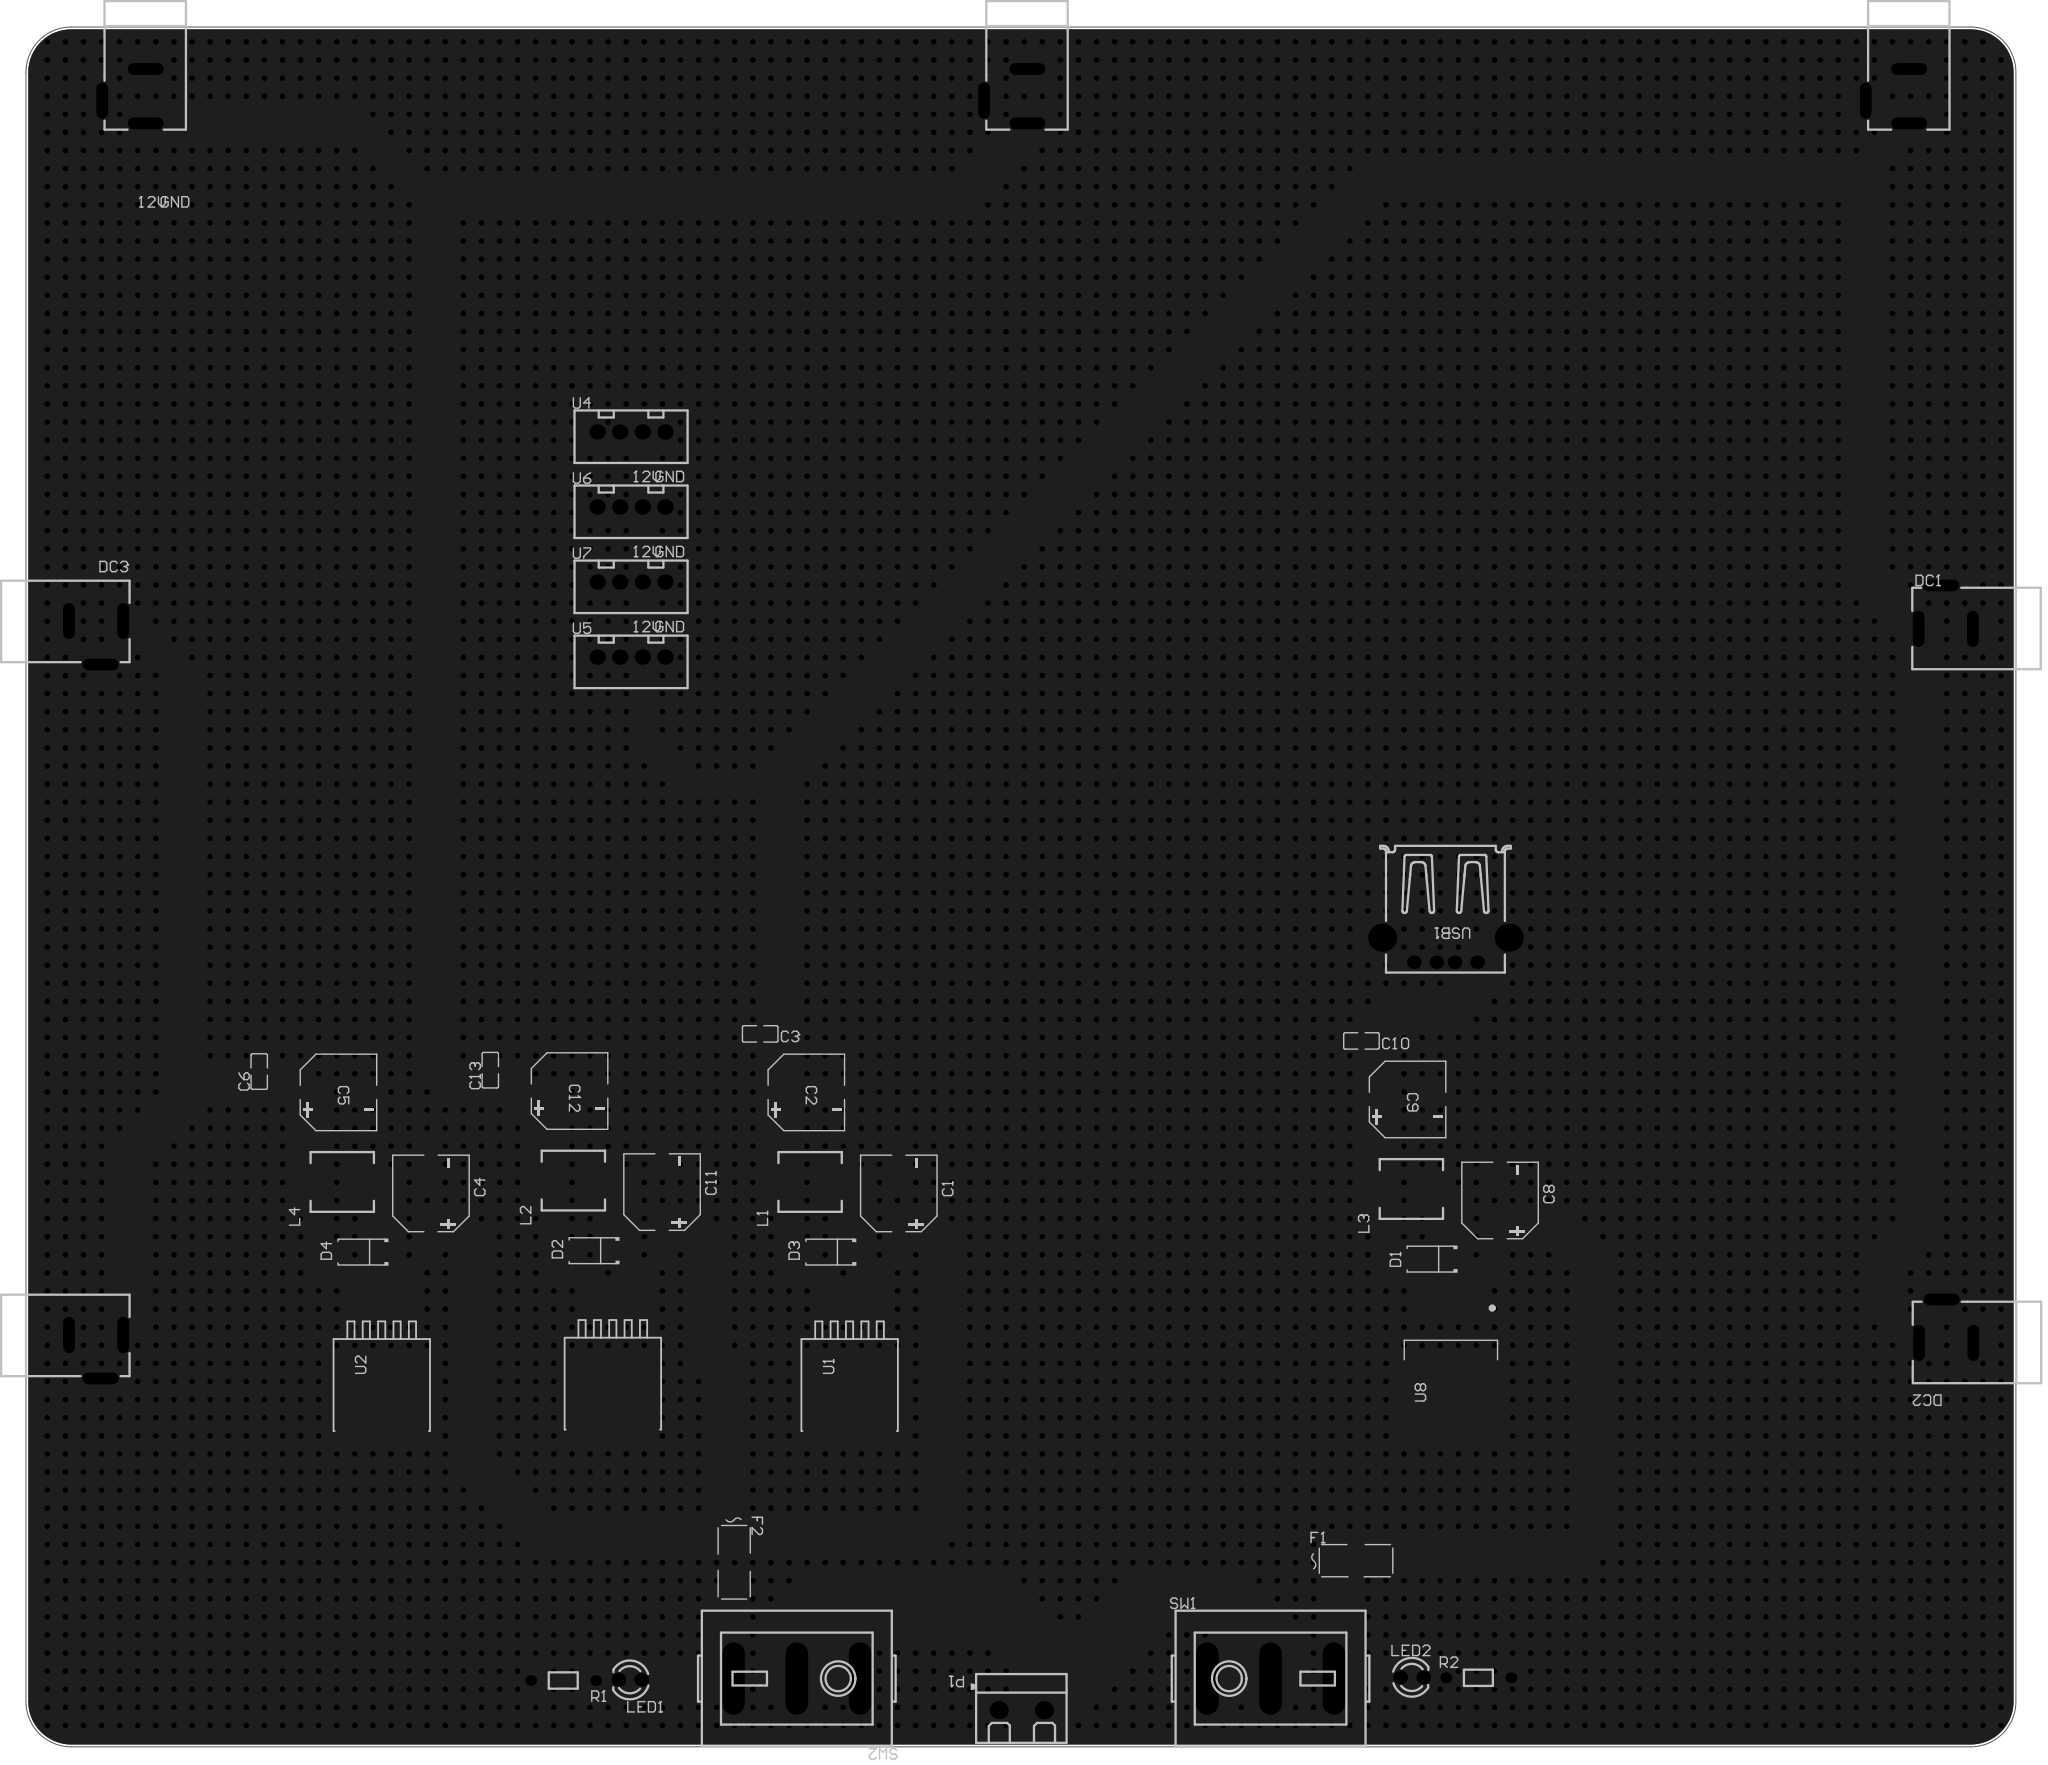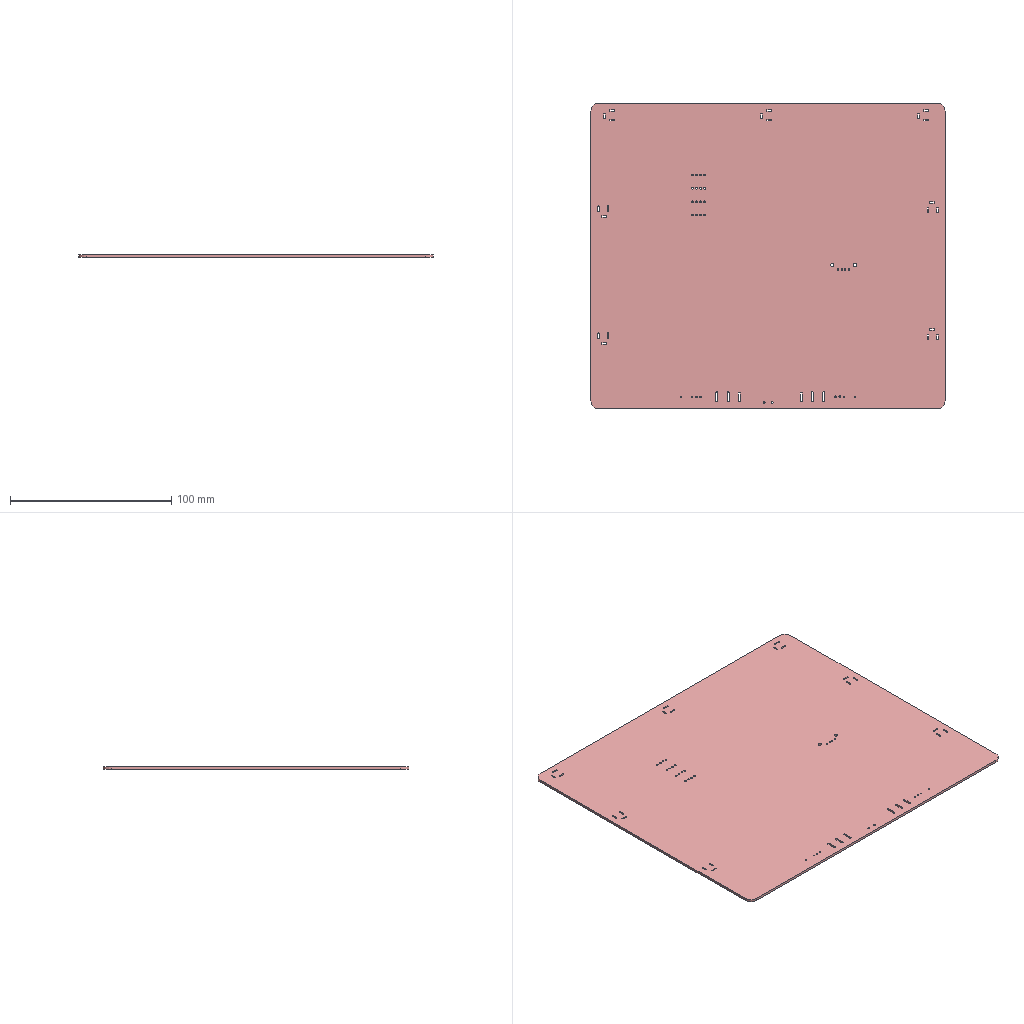Circuit board layout | Altium Designer | box 220 x 190 x 1.6 mm
Layer stack:
# Altium Designer layer stack of  (unit mm; dielectric type: 0 none, 1 core, 2 prepreg, 3 surface material)
index,name,kind,layer,copper_thickness_mm,dielectric_type,dielectric_thickness_mm,dielectric_material,dielectric_constant
0,Top Paste Mask Layer,other,,,,,,
1,Top Silkscreen Layer,other,,,,,,
2,Top Solder Mask Layer,dielectric,,,3,0.01,,3.3
3,Top Layer,copper,Top Layer,0.035,,,,
4,Dielectric1,dielectric,,,3,1.51,FR4,4.5
5,Bottom Layer,copper,Bottom Layer,0.035,,,,
6,Bottom Solder Mask Layer,dielectric,,,3,0.01,,3.3
7,Bottom Silkscreen Layer,other,,,,,,
8,Bottom Paste Mask Layer,other,,,,,,
# drill layer pairs: low layer,high layer
drill_pair,Top Layer,Bottom Layer
Part placement:
Designator,Comment,Layer,Footprint,Center-X(mm),Center-Y(mm),Rotation
L3,,TopLayer,IND-SMD_L7.0-W6.6,259.492,147.938,180
C8,,TopLayer,CAP-SMD_BD8.0-L8.3-W8.3-RD,269.296,146.668,270
C9,,TopLayer,CAP-SMD_BD8.0-L8.3-W8.3-RD,259.073,157.831,180
D1,,TopLayer,SMA_L4.3-W2.6-LS5.2-RD,261.626,140.191,180
C10,,TopLayer,C0805,253.973,164.296,180
L2,,TopLayer,IND-SMD_L7.0-W6.6,166.844,148.867,180
C11,,TopLayer,CAP-SMD_BD8.0-L8.3-W8.3-RD,176.648,147.597,270
C12,,TopLayer,CAP-SMD_BD8.0-L8.3-W8.3-RD,166.424,158.759,180
D2,,TopLayer,SMA_L4.3-W2.6-LS5.2-RD,168.977,141.12,180
C13,,TopLayer,C0805,157.661,161.064,90
U3,LM2596S-12,TopLayer,TO-263-5_L10.0-W8.4-P1.70-LS15.3-BR,171.213,130.262,90
U8,LM2596S-5.0,TopLayer,TO-263-5_L10.2-W8.9-P1.70-BR,263.861,129.723,90
DC2,,TopLayer,DC-2.0,318.623,133.337,0
DC3,,TopLayer,DC-2.0,114.077,208.288,180
P1,KF301-2P接线端子,TopLayer,CONN-TH_XY301V-A-5.0-2P,216.372,90.35,180
DC1,,TopLayer,DC-2.0,318.573,212.217,0
DC4,,TopLayer,DC-2.0,214.645,268.673,90
DC5,,TopLayer,DC-2.0,117.158,268.673,90
DC6,,TopLayer,DC-2.0,312.133,268.673,90
DC7,,TopLayer,DC-2.0,114.077,129.408,180
C1,,TopLayer,CAP-SMD_BD8.0-L8.3-W8.3-RD,202.823,147.447,270
C2,,TopLayer,CAP-SMD_BD8.0-L8.3-W8.3-RD,192.6,158.609,180
C3,,TopLayer,C0805,187.5,165.075,180
C4,,TopLayer,CAP-SMD_BD8.0-L8.3-W8.3-RD,151.098,147.447,270
C5,,TopLayer,CAP-SMD_BD8.0-L8.3-W8.3-RD,140.874,158.609,180
C6,,TopLayer,C0805,132.111,160.914,90
D3,,TopLayer,SMA_L4.3-W2.6-LS5.2-RD,195.153,140.97,180
D4,,TopLayer,SMA_L4.3-W2.6-LS5.2-RD,143.427,140.97,180
L1,,TopLayer,IND-SMD_L7.0-W6.6,193.019,148.717,180
L4,,TopLayer,IND-SMD_L7.0-W6.6,141.294,148.717,180
U1,LM2596S-12,TopLayer,TO-263-5_L10.0-W8.4-P1.70-LS15.3-BR,197.388,130.112,90
U2,LM2596S-12,TopLayer,TO-263-5_L10.0-W8.4-P1.70-LS15.3-BR,145.663,130.112,90
USB1,,TopLayer,USB__Type-A,263.259,174.344,180
SW1,船型开关601-10211BB,TopLayer,SW-TH_601-10211BB,243.925,93.85,0
SW2,船型开关601-10211BB,TopLayer,SW-TH_601-10211BB,191.55,93.85,180
U4,XH2.54_4P_直插,TopLayer,CONN-TH_4P-P2.50-XH2.54-4P,173.222,231.575,0
U5,XH2.54_4P_直插,TopLayer,CONN-TH_4P-P2.50-XH2.54-4P,173.222,206.7,0
U6,XH2.54_4P_直插,TopLayer,CONN-TH_4P-P2.50-XH2.54-4P,173.222,223.283,0
U7,XH2.54_4P_直插,TopLayer,CONN-TH_4P-P2.50-XH2.54-4P,173.222,214.992,0
F1,10A保险丝,TopLayer,FUSE-SMD_L6.1-W2.6,253.375,106.875,0
F2,10A保险丝,TopLayer,FUSE-SMD_L6.1-W2.6,184.625,106.7,270
LED1,,TopLayer,LED_TH-3mm,173.085,93.72,180
LED2,,TopLayer,LED_TH-3mm,259.539,93.978,0
R1,1kΩ,TopLayer,Res_1/8W,165.725,93.637,180
R2,1kΩ,TopLayer,Res_1/8W,266.9,93.938,0
Pad and via stacks:
# Altium Designer via and pad stacks of  (unit mm). Each distinct definition once, with the count of objects using it.
# via: kind,start_layer,end_layer,hole_mm,diameter_mm,mode(0 simple;1 top-mid-bottom;2 full stack),diameter_per_layer,count,example_net
# pad: kind,layer,hole_mm,hole_type(0 round;1 square;2 slot),plating,top_size,top_shape(1 round;2 rect;3 octagon;9 rounded rect),mid_size,bottom_size,mode,footprint,size_per_layer,count,example
pad,Top Layer,0,0,plated,2.799x3.701,2,2.799x3.701,2.799x3.701,0,IND-SMD_L7.0-W6.6,,8,L3.1
pad,Top Layer,0,0,plated,3.61x1.26,2,3.61x1.26,3.61x1.26,0,CAP-SMD_BD8.0-L8.3-W8.3-RD,,16,C8.1
pad,Top Layer,0,0,plated,2x2,2,2x2,2x2,0,SMA_L4.3-W2.6-LS5.2-RD,,8,D1.2
pad,Top Layer,0,0,plated,1.41x1.35,2,1.41x1.35,1.41x1.35,0,C0805,,8,C10.2
pad,Top Layer,0,0,plated,4x1.02,2,4x1.02,4x1.02,0,TO-263-5_L10.0-W8.4-P1.70-LS15.3-BR,,15,U3.1
pad,Top Layer,0,0,plated,8.4x10,2,8.4x10,8.4x10,0,TO-263-5_L10.0-W8.4-P1.70-LS15.3-BR,,3,U3.6
pad,Top Layer,0,0,plated,3.083x1.02,2,3.083x1.02,3.083x1.02,0,TO-263-5_L10.2-W8.9-P1.70-BR,,5,U8.1
pad,Top Layer,0,0,plated,8.5x11,2,8.5x11,8.5x11,0,TO-263-5_L10.2-W8.9-P1.70-BR,,1,U8.6
pad,Top Layer,0,0,plated,2.91x2.911,2,2.91x2.911,2.91x2.911,0,FUSE-SMD_L6.1-W2.6,,4,F1.2
pad,Multi-Layer,0.8001,2,plated,4x1.3,1,4x1.3,4x1.3,0,DC-2.0,,21,DC2.2
pad,Multi-Layer,1.2,0,plated,2x2,1,2x2,2x2,0,CONN-TH_XY301V-A-5.0-2P,,2,P1.1
pad,Multi-Layer,2.1,0,plated,3.1x3.1,1,3.1x3.1,3.1x3.1,0,USB_ Type-A,,2,USB1.SH2
pad,Multi-Layer,0.9,0,plated,1.5x1.5,1,1.5x1.5,1.5x1.5,0,USB_ Type-A,,4,USB1.1
pad,Multi-Layer,1.2,2,plated,8x2.5,1,8x2.5,8x2.5,0,SW-TH_601-10211BB,,6,SW1.1
pad,Multi-Layer,1.05,0,plated,1.7x1.7,1,1.7x1.7,1.7x1.7,0,CONN-TH_4P-P2.50-XH2.54-4P,,16,U4.1
pad,Multi-Layer,0.9144,0,plated,1.524x1.524,1,1.524x1.524,1.524x1.524,0,LED_TH-3mm,,4,LED1.1
pad,Multi-Layer,0.8001,0,plated,1.199x1.199,1,1.199x1.199,1.199x1.199,0,Res_1/8W,,4,R1.1
via,Top Layer,Bottom Layer,0.3048,0.61,0,,8689,GND
Copper pours:
name,layer,net,type(0 solid;1 hatched;2 none)
Top Layer-GND,Top Layer,GND,0
Bottom Layer-GND,Bottom Layer,GND,0
Design rules, without the lines most boards share:
# Altium Designer design rules of  (exported by Altium Designer, unit mm)
# columns: name | kind | enabled | priority | scope1 | scope2 | descriptor | typed fields (field=value)
otherClearance | 52 | enabled | 1 | All | All | Hole To Hole Clearance (Gap=11.8mil) (All),(All) | gap=0.2997
copperThickness1oz_2 | 2 | enabled | 2 | All | All | Width Constraint (Min=5mil) (Max=236.2mil) (Preferred=10mil) (All) |
copperRegion | 20 | enabled | 1 | All | All | Polygon Connect Rule(Relief Connect )(Conductor Width=39.37mil) (Relief Angle=45 Angle) (Entries=4) (Air Gap Width=10mil) (All),(All) | connect_style(0=relief,1=direct,2=none)=0 relief_conductor_width=1 relief_entries=4
solderMaskExpansion | 13 | enabled | 2 | All | All | Solder Mask Expansion (Expansion =2.008mil) (All) | expansion=0.051